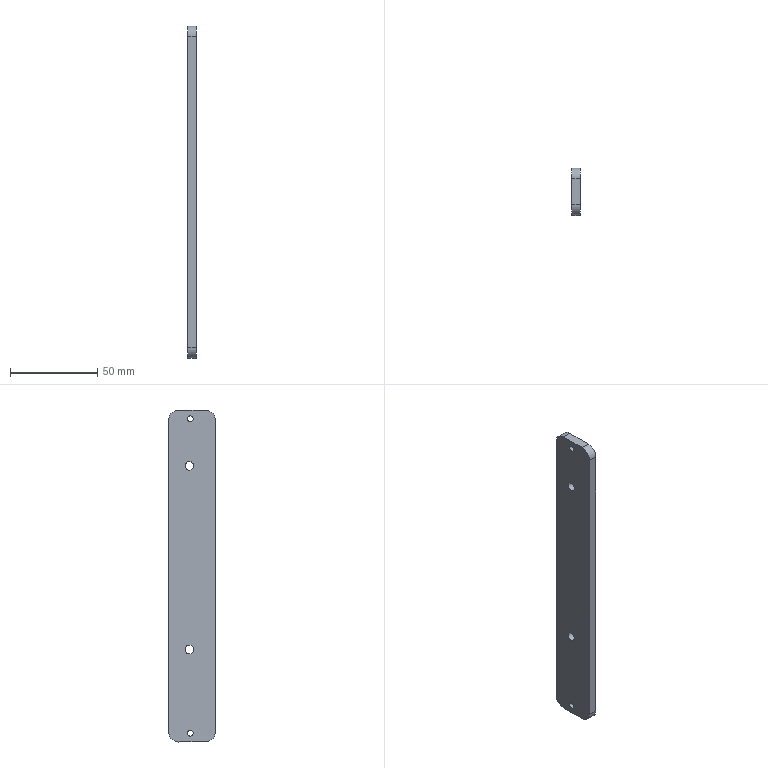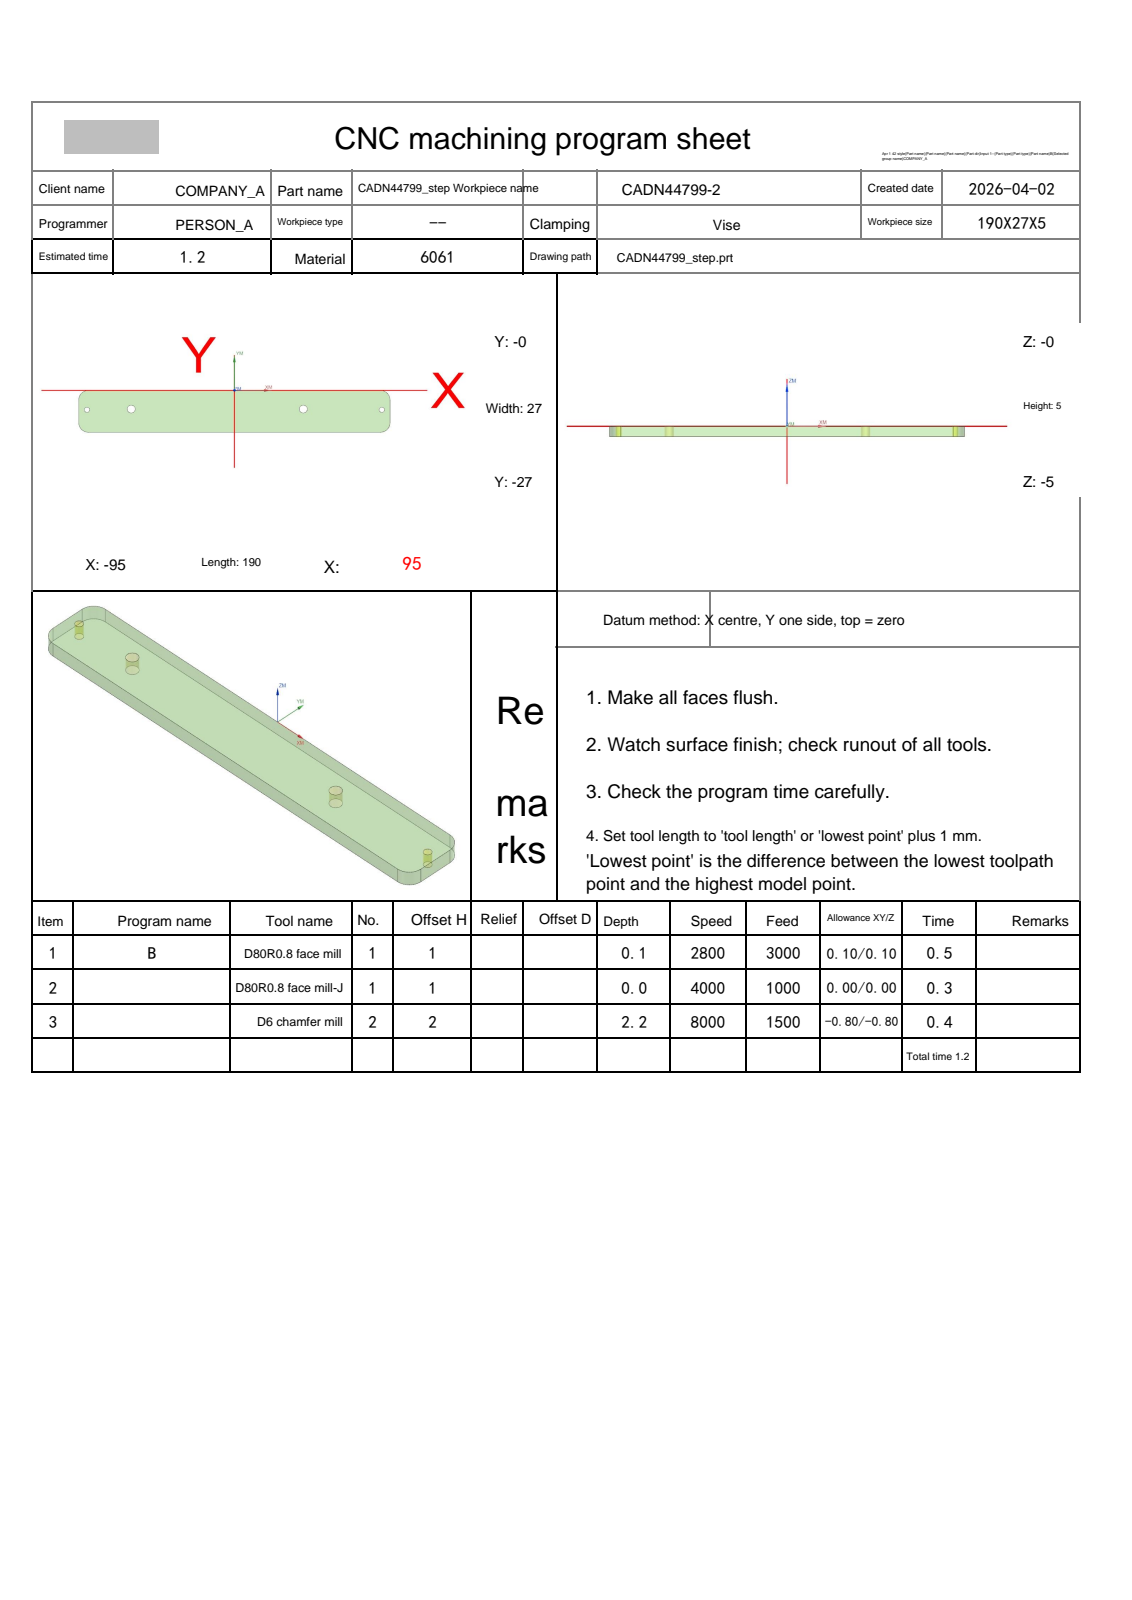NC program | NX | posted by the shop | part box 5 x 27 x 190 mm
Whole program:
%
O0001
(Machine time: 1.82 MIN)
(===Total Tool:2===)
(T1=D80R0.8 face mill D=80.  R=0.8  D-  H01 Z=0.    )
(T2=D6 chamfer mill   D=6.   R=0.   D-  H02 Z=-2.2  )
G80 G90 G17 G49 G40
G91 G28 Z0
M01
N1 T01 M06
(D80R0.8 face mill  D=80. R=0.8 H=01 ce=0.10 di=0.10)
G00 G90 G54 X-147.097 Y-13.503 M03 S2800
G43 H01 Z20.
M08
Z3.525
G01 Z1.525 F3000.
X-135.097
X135.097 Y-13.497
X147.097
Z3.525
G00 X-147.097 Y-13.503
Z3.05
G01 Z1.05
X-135.097
X135.097 Y-13.497
X147.097
Z3.05
G00 X-147.097 Y-13.503
Z2.575
G01 Z.575
X-135.097
X135.097 Y-13.497
X147.097
Z2.575
G00 X-147.097 Y-13.503
Z2.1
G01 Z.1
X-135.097
X135.097 Y-13.497
X147.097
Z2.1
G00 Z20.
G91 G28 Z0.0
M05
M09
G91 G28 Z0.0
M01
N2 T01 M06
(D80R0.8 face mill-J  D=80. R=0.8 H=01 ce=0.00 di=0.00)
G00 G90 G54 X-146.999 Y-13.5 M03 S4000
G43 H01 Z20.
M08
Z2.
G01 Z0.0 F1000.
X-134.999
X134.999
X146.999
Z2.
G00 Z20.
G91 G28 Z0.0
M05
M09
G91 G28 Z0.0
M01
N3 T02 M06
(D6 chamfer mill  D=6. R=0. H=02 ce=0.00 di=0.00)
G00 G90 G54 X-90.005 Y-12.5 M03 S8000
G43 H02 Z20.
M08
G98 G81 X-90.005 Y-12.5 Z-2.2 R3. F1000.
X89.995
G80
G00 Z20.
G00 G90 X41.812 Y-11.177 M03 S8000
Z20.
Z-.9
G01 Z-1.4 F600.
X41.643 Y-10.546
G03 X40.143 Y-12.046 I0.0 J-1.5
X42.043 Y-13.946 I1.9 J0.0
X43.943 Y-12.046 I0.0 J1.9
X42.043 Y-10.146 I-1.9 J0.0
X40.143 Y-12.046 I0.0 J-1.9
X41.643 Y-13.546 I1.5 J0.0
G01 X41.812 Y-12.916
Z-.9
G00 Z20.
X-63.233 Y-11.177
Z-.9
G01 Z-1.4
X-63.401 Y-10.546
G03 X-64.901 Y-12.046 I0.0 J-1.5
X-63.001 Y-13.946 I1.9 J0.0
X-61.101 Y-12.046 I0.0 J1.9
X-63.001 Y-10.146 I-1.9 J0.0
X-64.901 Y-12.046 I0.0 J-1.9
X-63.401 Y-13.546 I1.5 J0.0
G01 X-63.233 Y-12.916
Z-.9
G00 Z20.
G00 G90 X95.7 Y-11.384 M03 S7000
Z20.
Z2.5
G01 Y-21. Z-1. F1500.
G02 X89. Y-27.7 I-6.7 J0.0
G01 X-89.
G02 X-95.7 Y-21. I0.0 J6.7
G01 Y-6.
G02 X-89. Y.7 I6.7 J0.0
G01 X89.
G02 X95.7 Y-6. I0.0 J-6.7
G01 Y-21.
G02 X95.681 Y-21.5 I-6.7 J0.0
G01 Z1.5
G00 Z20.
M05
M09
G91 G28 Z0.0
G91 G28 Y0.0
M30
%